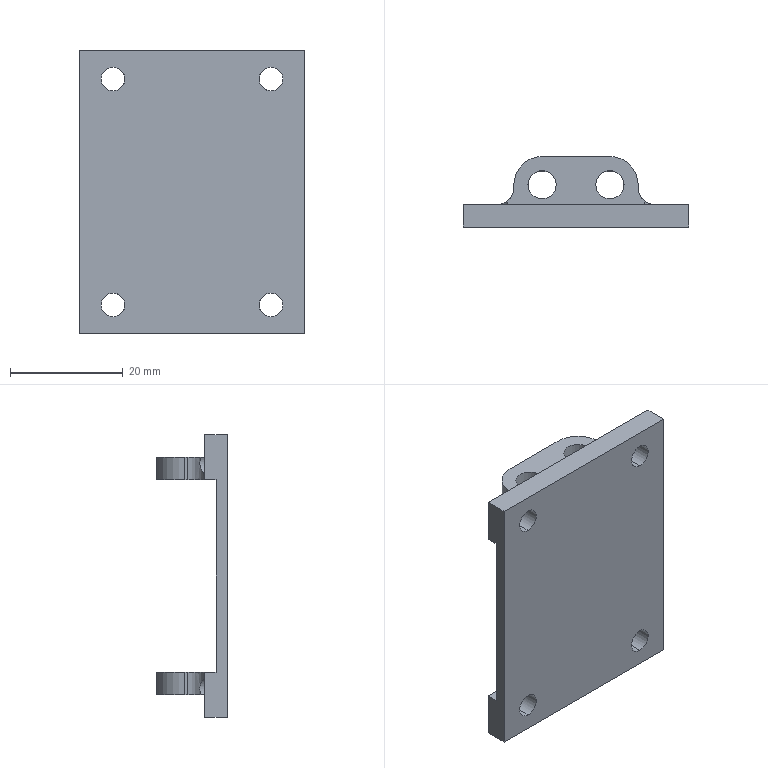Part | SolidWorks | features HoleWzd 3, ICE 3, Fillet 2, Extrusion 1 | 1 solid | 42 faces | box 40 x 12.5 x 50 mm | volume 6181 mm3 | cylinder 24 | plane 18 | commonest cylinder face diameters 4.2 x8 5 x8 6 x4 10 x4
STEP:
#1=CARTESIAN_POINT('',(2.5,0.,3.));
#2=VERTEX_POINT('',#1);
#3=CARTESIAN_POINT('',(-2.5,0.,3.));
#4=VERTEX_POINT('',#3);
#5=CARTESIAN_POINT('',(0.,0.,3.));
#6=DIRECTION('',(0.,0.,-1.));
#7=DIRECTION('',(-1.,0.,0.));
#8=AXIS2_PLACEMENT_3D('',#5,#6,#7);
#9=CIRCLE('',#8,2.5);
#10=EDGE_CURVE('',#2,#4,#9,.T.);
#11=ORIENTED_EDGE('',*,*,#10,.F.);
#12=CARTESIAN_POINT('',(2.5,0.,-1.));
#13=VERTEX_POINT('',#12);
#14=CARTESIAN_POINT('',(2.5,0.,-1.));
#15=DIRECTION('',(0.,0.,-1.));
#16=VECTOR('',#15,1000.);
#17=LINE('',#14,#16);
#18=EDGE_CURVE('',#2,#13,#17,.T.);
#19=ORIENTED_EDGE('',*,*,#18,.T.);
#20=CARTESIAN_POINT('',(-2.5,0.,-1.));
#21=VERTEX_POINT('',#20);
#22=CARTESIAN_POINT('',(0.,0.,-1.));
#23=DIRECTION('',(0.,0.,-1.));
#24=DIRECTION('',(-1.,0.,0.));
#25=AXIS2_PLACEMENT_3D('',#22,#23,#24);
#26=CIRCLE('',#25,2.5);
#27=EDGE_CURVE('',#13,#21,#26,.T.);
#28=ORIENTED_EDGE('',*,*,#27,.T.);
#29=CARTESIAN_POINT('',(-2.5,0.,-1.));
#30=DIRECTION('',(0.,0.,-1.));
#31=VECTOR('',#30,1000.);
#32=LINE('',#29,#31);
#33=EDGE_CURVE('',#4,#21,#32,.T.);
#34=ORIENTED_EDGE('',*,*,#33,.F.);
#35=EDGE_LOOP('',(#11,#19,#28,#34));
#36=FACE_OUTER_BOUND('',#35,.T.);
#37=CARTESIAN_POINT('',(0.,0.,-1.));
#38=DIRECTION('',(0.,0.,-1.));
#39=DIRECTION('',(-1.,0.,0.));
#40=AXIS2_PLACEMENT_3D('',#37,#38,#39);
#41=CYLINDRICAL_SURFACE('',#40,2.5);
#42=ADVANCED_FACE('',(#36),#41,.F.);
#43=CARTESIAN_POINT('',(14.5,0.,3.));
#44=VERTEX_POINT('',#43);
#45=CARTESIAN_POINT('',(9.5,0.,3.));
#46=VERTEX_POINT('',#45);
#47=CARTESIAN_POINT('',(12.,0.,3.));
#48=DIRECTION('',(0.,0.,-1.));
#49=DIRECTION('',(-1.,0.,0.));
#50=AXIS2_PLACEMENT_3D('',#47,#48,#49);
#51=CIRCLE('',#50,2.5);
#52=EDGE_CURVE('',#44,#46,#51,.T.);
#53=ORIENTED_EDGE('',*,*,#52,.F.);
#54=CARTESIAN_POINT('',(14.5,0.,-1.));
#55=VERTEX_POINT('',#54);
#56=CARTESIAN_POINT('',(14.5,0.,-1.));
#57=DIRECTION('',(0.,0.,-1.));
#58=VECTOR('',#57,1000.);
#59=LINE('',#56,#58);
#60=EDGE_CURVE('',#44,#55,#59,.T.);
#61=ORIENTED_EDGE('',*,*,#60,.T.);
#62=CARTESIAN_POINT('',(9.5,0.,-1.));
#63=VERTEX_POINT('',#62);
#64=CARTESIAN_POINT('',(12.,0.,-1.));
#65=DIRECTION('',(0.,0.,-1.));
#66=DIRECTION('',(-1.,0.,0.));
#67=AXIS2_PLACEMENT_3D('',#64,#65,#66);
#68=CIRCLE('',#67,2.5);
#69=EDGE_CURVE('',#55,#63,#68,.T.);
#70=ORIENTED_EDGE('',*,*,#69,.T.);
#71=CARTESIAN_POINT('',(9.5,0.,-1.));
#72=DIRECTION('',(0.,0.,-1.));
#73=VECTOR('',#72,1000.);
#74=LINE('',#71,#73);
#75=EDGE_CURVE('',#46,#63,#74,.T.);
#76=ORIENTED_EDGE('',*,*,#75,.F.);
#77=EDGE_LOOP('',(#53,#61,#70,#76));
#78=FACE_OUTER_BOUND('',#77,.T.);
#79=CARTESIAN_POINT('',(12.,0.,-1.));
#80=DIRECTION('',(0.,0.,-1.));
#81=DIRECTION('',(-1.,0.,0.));
#82=AXIS2_PLACEMENT_3D('',#79,#80,#81);
#83=CYLINDRICAL_SURFACE('',#82,2.5);
#84=ADVANCED_FACE('',(#78),#83,.F.);
#85=CARTESIAN_POINT('',(2.5,0.,41.));
#86=VERTEX_POINT('',#85);
#87=CARTESIAN_POINT('',(-2.5,0.,41.));
#88=VERTEX_POINT('',#87);
#89=CARTESIAN_POINT('',(0.,0.,41.));
#90=DIRECTION('',(0.,0.,-1.));
#91=DIRECTION('',(-1.,0.,0.));
#92=AXIS2_PLACEMENT_3D('',#89,#90,#91);
#93=CIRCLE('',#92,2.5);
#94=EDGE_CURVE('',#86,#88,#93,.T.);
#95=ORIENTED_EDGE('',*,*,#94,.F.);
#96=CARTESIAN_POINT('',(2.5,0.,37.));
#97=VERTEX_POINT('',#96);
#98=CARTESIAN_POINT('',(2.5,0.,37.));
#99=DIRECTION('',(0.,0.,-1.));
#100=VECTOR('',#99,1000.);
#101=LINE('',#98,#100);
#102=EDGE_CURVE('',#86,#97,#101,.T.);
#103=ORIENTED_EDGE('',*,*,#102,.T.);
#104=CARTESIAN_POINT('',(-2.5,0.,37.));
#105=VERTEX_POINT('',#104);
#106=CARTESIAN_POINT('',(0.,0.,37.));
#107=DIRECTION('',(0.,0.,-1.));
#108=DIRECTION('',(-1.,0.,0.));
#109=AXIS2_PLACEMENT_3D('',#106,#107,#108);
#110=CIRCLE('',#109,2.5);
#111=EDGE_CURVE('',#97,#105,#110,.T.);
#112=ORIENTED_EDGE('',*,*,#111,.T.);
#113=CARTESIAN_POINT('',(-2.5,0.,37.));
#114=DIRECTION('',(0.,0.,-1.));
#115=VECTOR('',#114,1000.);
#116=LINE('',#113,#115);
#117=EDGE_CURVE('',#88,#105,#116,.T.);
#118=ORIENTED_EDGE('',*,*,#117,.F.);
#119=EDGE_LOOP('',(#95,#103,#112,#118));
#120=FACE_OUTER_BOUND('',#119,.T.);
#121=CARTESIAN_POINT('',(0.,0.,37.));
#122=DIRECTION('',(0.,0.,-1.));
#123=DIRECTION('',(-1.,0.,0.));
#124=AXIS2_PLACEMENT_3D('',#121,#122,#123);
#125=CYLINDRICAL_SURFACE('',#124,2.5);
#126=ADVANCED_FACE('',(#120),#125,.F.);
#127=CARTESIAN_POINT('',(14.5,0.,41.));
#128=VERTEX_POINT('',#127);
#129=CARTESIAN_POINT('',(9.5,0.,41.));
#130=VERTEX_POINT('',#129);
#131=CARTESIAN_POINT('',(12.,0.,41.));
#132=DIRECTION('',(0.,0.,-1.));
#133=DIRECTION('',(-1.,0.,0.));
#134=AXIS2_PLACEMENT_3D('',#131,#132,#133);
#135=CIRCLE('',#134,2.5);
#136=EDGE_CURVE('',#128,#130,#135,.T.);
#137=ORIENTED_EDGE('',*,*,#136,.F.);
#138=CARTESIAN_POINT('',(14.5,0.,37.));
#139=VERTEX_POINT('',#138);
#140=CARTESIAN_POINT('',(14.5,0.,37.));
#141=DIRECTION('',(0.,0.,-1.));
#142=VECTOR('',#141,1000.);
#143=LINE('',#140,#142);
#144=EDGE_CURVE('',#128,#139,#143,.T.);
#145=ORIENTED_EDGE('',*,*,#144,.T.);
#146=CARTESIAN_POINT('',(9.5,0.,37.));
#147=VERTEX_POINT('',#146);
#148=CARTESIAN_POINT('',(12.,0.,37.));
#149=DIRECTION('',(0.,0.,-1.));
#150=DIRECTION('',(-1.,0.,0.));
#151=AXIS2_PLACEMENT_3D('',#148,#149,#150);
#152=CIRCLE('',#151,2.5);
#153=EDGE_CURVE('',#139,#147,#152,.T.);
#154=ORIENTED_EDGE('',*,*,#153,.T.);
#155=CARTESIAN_POINT('',(9.5,0.,37.));
#156=DIRECTION('',(0.,0.,-1.));
#157=VECTOR('',#156,1000.);
#158=LINE('',#155,#157);
#159=EDGE_CURVE('',#130,#147,#158,.T.);
#160=ORIENTED_EDGE('',*,*,#159,.F.);
#161=EDGE_LOOP('',(#137,#145,#154,#160));
#162=FACE_OUTER_BOUND('',#161,.T.);
#163=CARTESIAN_POINT('',(12.,0.,37.));
#164=DIRECTION('',(0.,0.,-1.));
#165=DIRECTION('',(-1.,0.,0.));
#166=AXIS2_PLACEMENT_3D('',#163,#164,#165);
#167=CYLINDRICAL_SURFACE('',#166,2.5);
#168=ADVANCED_FACE('',(#162),#167,.F.);
#169=CARTESIAN_POINT('',(18.153,-3.5,41.));
#170=VERTEX_POINT('',#169);
#171=CARTESIAN_POINT('',(20.,-3.5,42.1));
#172=VERTEX_POINT('',#171);
#173=CARTESIAN_POINT('',(20.,-3.5,40.));
#174=DIRECTION('',(0.,1.,0.));
#175=DIRECTION('',(0.,0.,1.));
#176=AXIS2_PLACEMENT_3D('',#173,#174,#175);
#177=CIRCLE('',#176,2.1);
#178=EDGE_CURVE('',#170,#172,#177,.T.);
#179=ORIENTED_EDGE('',*,*,#178,.T.);
#180=CARTESIAN_POINT('',(20.,-7.5,42.1));
#181=VERTEX_POINT('',#180);
#182=CARTESIAN_POINT('',(20.,-7.5,42.1));
#183=DIRECTION('',(0.,-1.,0.));
#184=VECTOR('',#183,1000.);
#185=LINE('',#182,#184);
#186=EDGE_CURVE('',#172,#181,#185,.T.);
#187=ORIENTED_EDGE('',*,*,#186,.T.);
#188=CARTESIAN_POINT('',(20.,-7.5,37.9));
#189=VERTEX_POINT('',#188);
#190=CARTESIAN_POINT('',(20.,-7.5,40.));
#191=DIRECTION('',(0.,-1.,0.));
#192=DIRECTION('',(0.,0.,-1.));
#193=AXIS2_PLACEMENT_3D('',#190,#191,#192);
#194=CIRCLE('',#193,2.1);
#195=EDGE_CURVE('',#181,#189,#194,.T.);
#196=ORIENTED_EDGE('',*,*,#195,.T.);
#197=CARTESIAN_POINT('',(20.,-3.5,37.9));
#198=VERTEX_POINT('',#197);
#199=CARTESIAN_POINT('',(20.,-7.5,37.9));
#200=DIRECTION('',(0.,-1.,0.));
#201=VECTOR('',#200,1000.);
#202=LINE('',#199,#201);
#203=EDGE_CURVE('',#198,#189,#202,.T.);
#204=ORIENTED_EDGE('',*,*,#203,.F.);
#205=CARTESIAN_POINT('',(18.153,-2.864,41.));
#206=VERTEX_POINT('',#205);
#207=CARTESIAN_POINT('',(20.,-3.5,37.9));
#208=CARTESIAN_POINT('',(19.811,-3.5,37.9));
#209=CARTESIAN_POINT('',(19.627,-3.482,37.925));
#210=CARTESIAN_POINT('',(19.269,-3.415,38.023));
#211=CARTESIAN_POINT('',(19.101,-3.367,38.094));
#212=CARTESIAN_POINT('',(18.638,-3.193,38.362));
#213=CARTESIAN_POINT('',(18.385,-3.038,38.614));
#214=CARTESIAN_POINT('',(18.115,-2.836,39.059));
#215=CARTESIAN_POINT('',(18.041,-2.773,39.222));
#216=CARTESIAN_POINT('',(17.963,-2.702,39.483));
#217=CARTESIAN_POINT('',(17.942,-2.683,39.573));
#218=CARTESIAN_POINT('',(17.912,-2.654,39.755));
#219=CARTESIAN_POINT('',(17.903,-2.646,39.85));
#220=CARTESIAN_POINT('',(17.896,-2.638,40.132));
#221=CARTESIAN_POINT('',(17.916,-2.659,40.319));
#222=CARTESIAN_POINT('',(18.004,-2.74,40.677));
#223=CARTESIAN_POINT('',(18.07,-2.799,40.845));
#224=CARTESIAN_POINT('',(18.153,-2.864,41.));
#225=B_SPLINE_CURVE_WITH_KNOTS('',3,(#207,#208,#209,#210,#211,#212,#213,#214,#215,#216,#217,#218,#219,#220,#221,#222,#223,#224),.UNSPECIFIED.,.F.,.F.,(4,2,2,2,2,2,2,2,4),(0.,0.0005592,0.001118,0.002237,0.002796,0.003076,0.003355,0.003915,0.004474),.UNSPECIFIED.);
#226=EDGE_CURVE('',#198,#206,#225,.T.);
#227=ORIENTED_EDGE('',*,*,#226,.T.);
#228=CARTESIAN_POINT('',(18.153,-2.864,41.));
#229=DIRECTION('',(0.,1.,0.));
#230=VECTOR('',#229,1000.);
#231=LINE('',#228,#230);
#232=EDGE_CURVE('',#170,#206,#231,.T.);
#233=ORIENTED_EDGE('',*,*,#232,.F.);
#234=EDGE_LOOP('',(#179,#187,#196,#204,#227,#233));
#235=FACE_OUTER_BOUND('',#234,.T.);
#236=CARTESIAN_POINT('',(20.,-7.5,40.));
#237=DIRECTION('',(0.,-1.,0.));
#238=DIRECTION('',(0.,0.,-1.));
#239=AXIS2_PLACEMENT_3D('',#236,#237,#238);
#240=CYLINDRICAL_SURFACE('',#239,2.1);
#241=ADVANCED_FACE('',(#235),#240,.F.);
#242=CARTESIAN_POINT('',(18.153,-2.864,-1.));
#243=VERTEX_POINT('',#242);
#244=CARTESIAN_POINT('',(20.,-3.5,2.1));
#245=VERTEX_POINT('',#244);
#246=CARTESIAN_POINT('',(18.153,-2.864,-1.));
#247=CARTESIAN_POINT('',(18.07,-2.799,-0.8455));
#248=CARTESIAN_POINT('',(18.004,-2.74,-0.6767));
#249=CARTESIAN_POINT('',(17.916,-2.659,-0.3194));
#250=CARTESIAN_POINT('',(17.896,-2.638,-0.1317));
#251=CARTESIAN_POINT('',(17.903,-2.646,0.15));
#252=CARTESIAN_POINT('',(17.912,-2.654,0.2446));
#253=CARTESIAN_POINT('',(17.942,-2.683,0.4274));
#254=CARTESIAN_POINT('',(17.963,-2.702,0.5166));
#255=CARTESIAN_POINT('',(18.041,-2.773,0.7784));
#256=CARTESIAN_POINT('',(18.115,-2.836,0.9408));
#257=CARTESIAN_POINT('',(18.385,-3.038,1.386));
#258=CARTESIAN_POINT('',(18.638,-3.193,1.638));
#259=CARTESIAN_POINT('',(19.101,-3.367,1.906));
#260=CARTESIAN_POINT('',(19.269,-3.415,1.977));
#261=CARTESIAN_POINT('',(19.627,-3.482,2.075));
#262=CARTESIAN_POINT('',(19.811,-3.5,2.1));
#263=CARTESIAN_POINT('',(20.,-3.5,2.1));
#264=B_SPLINE_CURVE_WITH_KNOTS('',3,(#246,#247,#248,#249,#250,#251,#252,#253,#254,#255,#256,#257,#258,#259,#260,#261,#262,#263),.UNSPECIFIED.,.F.,.F.,(4,2,2,2,2,2,2,2,4),(0.0006281,0.001188,0.001748,0.002027,0.002307,0.002867,0.003986,0.004546,0.005106),.UNSPECIFIED.);
#265=EDGE_CURVE('',#243,#245,#264,.T.);
#266=ORIENTED_EDGE('',*,*,#265,.T.);
#267=CARTESIAN_POINT('',(20.,-7.5,2.1));
#268=VERTEX_POINT('',#267);
#269=CARTESIAN_POINT('',(20.,-7.5,2.1));
#270=DIRECTION('',(0.,-1.,0.));
#271=VECTOR('',#270,1000.);
#272=LINE('',#269,#271);
#273=EDGE_CURVE('',#245,#268,#272,.T.);
#274=ORIENTED_EDGE('',*,*,#273,.T.);
#275=CARTESIAN_POINT('',(20.,-7.5,-2.1));
#276=VERTEX_POINT('',#275);
#277=CARTESIAN_POINT('',(20.,-7.5,0.));
#278=DIRECTION('',(0.,-1.,0.));
#279=DIRECTION('',(0.,0.,-1.));
#280=AXIS2_PLACEMENT_3D('',#277,#278,#279);
#281=CIRCLE('',#280,2.1);
#282=EDGE_CURVE('',#268,#276,#281,.T.);
#283=ORIENTED_EDGE('',*,*,#282,.T.);
#284=CARTESIAN_POINT('',(20.,-3.5,-2.1));
#285=VERTEX_POINT('',#284);
#286=CARTESIAN_POINT('',(20.,-7.5,-2.1));
#287=DIRECTION('',(0.,-1.,0.));
#288=VECTOR('',#287,1000.);
#289=LINE('',#286,#288);
#290=EDGE_CURVE('',#285,#276,#289,.T.);
#291=ORIENTED_EDGE('',*,*,#290,.F.);
#292=CARTESIAN_POINT('',(18.153,-3.5,-1.));
#293=VERTEX_POINT('',#292);
#294=CARTESIAN_POINT('',(20.,-3.5,0.));
#295=DIRECTION('',(0.,1.,0.));
#296=DIRECTION('',(0.,0.,1.));
#297=AXIS2_PLACEMENT_3D('',#294,#295,#296);
#298=CIRCLE('',#297,2.1);
#299=EDGE_CURVE('',#285,#293,#298,.T.);
#300=ORIENTED_EDGE('',*,*,#299,.T.);
#301=CARTESIAN_POINT('',(18.153,-3.5,-1.));
#302=DIRECTION('',(0.,1.,0.));
#303=VECTOR('',#302,1000.);
#304=LINE('',#301,#303);
#305=EDGE_CURVE('',#293,#243,#304,.T.);
#306=ORIENTED_EDGE('',*,*,#305,.T.);
#307=EDGE_LOOP('',(#266,#274,#283,#291,#300,#306));
#308=FACE_OUTER_BOUND('',#307,.T.);
#309=CARTESIAN_POINT('',(20.,-7.5,0.));
#310=DIRECTION('',(0.,-1.,0.));
#311=DIRECTION('',(0.,0.,-1.));
#312=AXIS2_PLACEMENT_3D('',#309,#310,#311);
#313=CYLINDRICAL_SURFACE('',#312,2.1);
#314=ADVANCED_FACE('',(#308),#313,.F.);
#315=CARTESIAN_POINT('',(-8.,-3.5,-2.1));
#316=VERTEX_POINT('',#315);
#317=CARTESIAN_POINT('',(-8.,-3.5,2.1));
#318=VERTEX_POINT('',#317);
#319=CARTESIAN_POINT('',(-8.,-3.5,0.));
#320=DIRECTION('',(0.,1.,0.));
#321=DIRECTION('',(0.,0.,1.));
#322=AXIS2_PLACEMENT_3D('',#319,#320,#321);
#323=CIRCLE('',#322,2.1);
#324=EDGE_CURVE('',#316,#318,#323,.T.);
#325=ORIENTED_EDGE('',*,*,#324,.T.);
#326=CARTESIAN_POINT('',(-8.,-7.5,2.1));
#327=VERTEX_POINT('',#326);
#328=CARTESIAN_POINT('',(-8.,-7.5,2.1));
#329=DIRECTION('',(0.,-1.,0.));
#330=VECTOR('',#329,1000.);
#331=LINE('',#328,#330);
#332=EDGE_CURVE('',#318,#327,#331,.T.);
#333=ORIENTED_EDGE('',*,*,#332,.T.);
#334=CARTESIAN_POINT('',(-8.,-7.5,-2.1));
#335=VERTEX_POINT('',#334);
#336=CARTESIAN_POINT('',(-8.,-7.5,0.));
#337=DIRECTION('',(0.,-1.,0.));
#338=DIRECTION('',(0.,0.,-1.));
#339=AXIS2_PLACEMENT_3D('',#336,#337,#338);
#340=CIRCLE('',#339,2.1);
#341=EDGE_CURVE('',#327,#335,#340,.T.);
#342=ORIENTED_EDGE('',*,*,#341,.T.);
#343=CARTESIAN_POINT('',(-8.,-7.5,-2.1));
#344=DIRECTION('',(0.,-1.,0.));
#345=VECTOR('',#344,1000.);
#346=LINE('',#343,#345);
#347=EDGE_CURVE('',#316,#335,#346,.T.);
#348=ORIENTED_EDGE('',*,*,#347,.F.);
#349=EDGE_LOOP('',(#325,#333,#342,#348));
#350=FACE_OUTER_BOUND('',#349,.T.);
#351=CARTESIAN_POINT('',(-8.,-7.5,0.));
#352=DIRECTION('',(0.,-1.,0.));
#353=DIRECTION('',(0.,0.,-1.));
#354=AXIS2_PLACEMENT_3D('',#351,#352,#353);
#355=CYLINDRICAL_SURFACE('',#354,2.1);
#356=ADVANCED_FACE('',(#350),#355,.F.);
#357=CARTESIAN_POINT('',(-8.,-3.5,37.9));
#358=VERTEX_POINT('',#357);
#359=CARTESIAN_POINT('',(-8.,-3.5,42.1));
#360=VERTEX_POINT('',#359);
#361=CARTESIAN_POINT('',(-8.,-3.5,40.));
#362=DIRECTION('',(0.,1.,0.));
#363=DIRECTION('',(0.,0.,1.));
#364=AXIS2_PLACEMENT_3D('',#361,#362,#363);
#365=CIRCLE('',#364,2.1);
#366=EDGE_CURVE('',#358,#360,#365,.T.);
#367=ORIENTED_EDGE('',*,*,#366,.T.);
#368=CARTESIAN_POINT('',(-8.,-7.5,42.1));
#369=VERTEX_POINT('',#368);
#370=CARTESIAN_POINT('',(-8.,-7.5,42.1));
#371=DIRECTION('',(0.,-1.,0.));
#372=VECTOR('',#371,1000.);
#373=LINE('',#370,#372);
#374=EDGE_CURVE('',#360,#369,#373,.T.);
#375=ORIENTED_EDGE('',*,*,#374,.T.);
#376=CARTESIAN_POINT('',(-8.,-7.5,37.9));
#377=VERTEX_POINT('',#376);
#378=CARTESIAN_POINT('',(-8.,-7.5,40.));
#379=DIRECTION('',(0.,-1.,0.));
#380=DIRECTION('',(0.,0.,-1.));
#381=AXIS2_PLACEMENT_3D('',#378,#379,#380);
#382=CIRCLE('',#381,2.1);
#383=EDGE_CURVE('',#369,#377,#382,.T.);
#384=ORIENTED_EDGE('',*,*,#383,.T.);
#385=CARTESIAN_POINT('',(-8.,-7.5,37.9));
#386=DIRECTION('',(0.,-1.,0.));
#387=VECTOR('',#386,1000.);
#388=LINE('',#385,#387);
#389=EDGE_CURVE('',#358,#377,#388,.T.);
#390=ORIENTED_EDGE('',*,*,#389,.F.);
#391=EDGE_LOOP('',(#367,#375,#384,#390));
#392=FACE_OUTER_BOUND('',#391,.T.);
#393=CARTESIAN_POINT('',(-8.,-7.5,40.));
#394=DIRECTION('',(0.,-1.,0.));
#395=DIRECTION('',(0.,0.,-1.));
#396=AXIS2_PLACEMENT_3D('',#393,#394,#395);
#397=CYLINDRICAL_SURFACE('',#396,2.1);
#398=ADVANCED_FACE('',(#392),#397,.F.);
#399=CARTESIAN_POINT('',(-6.153,-3.5,41.));
#400=VERTEX_POINT('',#399);
#401=CARTESIAN_POINT('',(17.,-3.5,41.));
#402=DIRECTION('',(1.,0.,0.));
#403=VECTOR('',#402,1000.);
#404=LINE('',#401,#403);
#405=EDGE_CURVE('',#400,#170,#404,.T.);
#406=ORIENTED_EDGE('',*,*,#405,.F.);
#407=CARTESIAN_POINT('',(-8.,-3.5,40.));
#408=DIRECTION('',(0.,1.,0.));
#409=DIRECTION('',(0.,0.,1.));
#410=AXIS2_PLACEMENT_3D('',#407,#408,#409);
#411=CIRCLE('',#410,2.1);
#412=EDGE_CURVE('',#360,#400,#411,.T.);
#413=ORIENTED_EDGE('',*,*,#412,.F.);
#414=ORIENTED_EDGE('',*,*,#366,.F.);
#415=CARTESIAN_POINT('',(-8.,-3.5,37.));
#416=VERTEX_POINT('',#415);
#417=CARTESIAN_POINT('',(-8.,-3.5,0.));
#418=DIRECTION('',(0.,0.,-1.));
#419=VECTOR('',#418,1000.);
#420=LINE('',#417,#419);
#421=EDGE_CURVE('',#358,#416,#420,.T.);
#422=ORIENTED_EDGE('',*,*,#421,.T.);
#423=CARTESIAN_POINT('',(-14.,-3.5,37.));
#424=VERTEX_POINT('',#423);
#425=CARTESIAN_POINT('',(-14.,-3.5,37.));
#426=DIRECTION('',(1.,0.,0.));
#427=VECTOR('',#426,1000.);
#428=LINE('',#425,#427);
#429=EDGE_CURVE('',#424,#416,#428,.T.);
#430=ORIENTED_EDGE('',*,*,#429,.F.);
#431=CARTESIAN_POINT('',(-14.,-3.5,45.));
#432=VERTEX_POINT('',#431);
#433=CARTESIAN_POINT('',(-14.,-3.5,-5.));
#434=DIRECTION('',(0.,0.,1.));
#435=VECTOR('',#434,1000.);
#436=LINE('',#433,#435);
#437=EDGE_CURVE('',#424,#432,#436,.T.);
#438=ORIENTED_EDGE('',*,*,#437,.T.);
#439=CARTESIAN_POINT('',(26.,-3.5,45.));
#440=VERTEX_POINT('',#439);
#441=CARTESIAN_POINT('',(-14.,-3.5,45.));
#442=DIRECTION('',(1.,0.,0.));
#443=VECTOR('',#442,1000.);
#444=LINE('',#441,#443);
#445=EDGE_CURVE('',#432,#440,#444,.T.);
#446=ORIENTED_EDGE('',*,*,#445,.T.);
#447=CARTESIAN_POINT('',(26.,-3.5,37.));
#448=VERTEX_POINT('',#447);
#449=CARTESIAN_POINT('',(26.,-3.5,45.));
#450=DIRECTION('',(0.,0.,-1.));
#451=VECTOR('',#450,1000.);
#452=LINE('',#449,#451);
#453=EDGE_CURVE('',#440,#448,#452,.T.);
#454=ORIENTED_EDGE('',*,*,#453,.T.);
#455=CARTESIAN_POINT('',(20.,-3.5,37.));
#456=VERTEX_POINT('',#455);
#457=CARTESIAN_POINT('',(-14.,-3.5,37.));
#458=DIRECTION('',(1.,0.,0.));
#459=VECTOR('',#458,1000.);
#460=LINE('',#457,#459);
#461=EDGE_CURVE('',#456,#448,#460,.T.);
#462=ORIENTED_EDGE('',*,*,#461,.F.);
#463=CARTESIAN_POINT('',(20.,-3.5,0.));
#464=DIRECTION('',(0.,0.,1.));
#465=VECTOR('',#464,1000.);
#466=LINE('',#463,#465);
#467=EDGE_CURVE('',#456,#198,#466,.T.);
#468=ORIENTED_EDGE('',*,*,#467,.T.);
#469=CARTESIAN_POINT('',(20.,-3.5,40.));
#470=DIRECTION('',(0.,1.,0.));
#471=DIRECTION('',(0.,0.,1.));
#472=AXIS2_PLACEMENT_3D('',#469,#470,#471);
#473=CIRCLE('',#472,2.1);
#474=EDGE_CURVE('',#172,#198,#473,.T.);
#475=ORIENTED_EDGE('',*,*,#474,.F.);
#476=ORIENTED_EDGE('',*,*,#178,.F.);
#477=EDGE_LOOP('',(#406,#413,#414,#422,#430,#438,#446,#454,#462,#468,#475,#476));
#478=FACE_OUTER_BOUND('',#477,.T.);
#479=CARTESIAN_POINT('',(0.,-3.5,0.));
#480=DIRECTION('',(0.,1.,0.));
#481=DIRECTION('',(0.,0.,1.));
#482=AXIS2_PLACEMENT_3D('',#479,#480,#481);
#483=PLANE('',#482);
#484=ADVANCED_FACE('',(#478),#483,.T.);
#485=CARTESIAN_POINT('',(-14.,-3.5,3.));
#486=VERTEX_POINT('',#485);
#487=CARTESIAN_POINT('',(-8.,-3.5,3.));
#488=VERTEX_POINT('',#487);
#489=CARTESIAN_POINT('',(-14.,-3.5,3.));
#490=DIRECTION('',(1.,0.,0.));
#491=VECTOR('',#490,1000.);
#492=LINE('',#489,#491);
#493=EDGE_CURVE('',#486,#488,#492,.T.);
#494=ORIENTED_EDGE('',*,*,#493,.T.);
#495=CARTESIAN_POINT('',(-8.,-3.5,0.));
#496=DIRECTION('',(0.,0.,-1.));
#497=VECTOR('',#496,1000.);
#498=LINE('',#495,#497);
#499=EDGE_CURVE('',#488,#318,#498,.T.);
#500=ORIENTED_EDGE('',*,*,#499,.T.);
#501=ORIENTED_EDGE('',*,*,#324,.F.);
#502=CARTESIAN_POINT('',(-6.153,-3.5,-1.));
#503=VERTEX_POINT('',#502);
#504=CARTESIAN_POINT('',(-8.,-3.5,0.));
#505=DIRECTION('',(0.,1.,0.));
#506=DIRECTION('',(0.,0.,1.));
#507=AXIS2_PLACEMENT_3D('',#504,#505,#506);
#508=CIRCLE('',#507,2.1);
#509=EDGE_CURVE('',#503,#316,#508,.T.);
#510=ORIENTED_EDGE('',*,*,#509,.F.);
#511=CARTESIAN_POINT('',(-5.,-3.5,-1.));
#512=DIRECTION('',(-1.,0.,0.));
#513=VECTOR('',#512,1000.);
#514=LINE('',#511,#513);
#515=EDGE_CURVE('',#293,#503,#514,.T.);
#516=ORIENTED_EDGE('',*,*,#515,.F.);
#517=ORIENTED_EDGE('',*,*,#299,.F.);
#518=CARTESIAN_POINT('',(20.,-3.5,0.));
#519=DIRECTION('',(0.,1.,0.));
#520=DIRECTION('',(0.,0.,1.));
#521=AXIS2_PLACEMENT_3D('',#518,#519,#520);
#522=CIRCLE('',#521,2.1);
#523=EDGE_CURVE('',#245,#285,#522,.T.);
#524=ORIENTED_EDGE('',*,*,#523,.F.);
#525=CARTESIAN_POINT('',(20.,-3.5,3.));
#526=VERTEX_POINT('',#525);
#527=CARTESIAN_POINT('',(20.,-3.5,0.));
#528=DIRECTION('',(0.,0.,1.));
#529=VECTOR('',#528,1000.);
#530=LINE('',#527,#529);
#531=EDGE_CURVE('',#245,#526,#530,.T.);
#532=ORIENTED_EDGE('',*,*,#531,.T.);
#533=CARTESIAN_POINT('',(26.,-3.5,3.));
#534=VERTEX_POINT('',#533);
#535=CARTESIAN_POINT('',(-14.,-3.5,3.));
#536=DIRECTION('',(1.,0.,0.));
#537=VECTOR('',#536,1000.);
#538=LINE('',#535,#537);
#539=EDGE_CURVE('',#526,#534,#538,.T.);
#540=ORIENTED_EDGE('',*,*,#539,.T.);
#541=CARTESIAN_POINT('',(26.,-3.5,-5.));
#542=VERTEX_POINT('',#541);
#543=CARTESIAN_POINT('',(26.,-3.5,45.));
#544=DIRECTION('',(0.,0.,-1.));
#545=VECTOR('',#544,1000.);
#546=LINE('',#543,#545);
#547=EDGE_CURVE('',#534,#542,#546,.T.);
#548=ORIENTED_EDGE('',*,*,#547,.T.);
#549=CARTESIAN_POINT('',(-14.,-3.5,-5.));
#550=VERTEX_POINT('',#549);
#551=CARTESIAN_POINT('',(26.,-3.5,-5.));
#552=DIRECTION('',(-1.,0.,0.));
#553=VECTOR('',#552,1000.);
#554=LINE('',#551,#553);
#555=EDGE_CURVE('',#542,#550,#554,.T.);
#556=ORIENTED_EDGE('',*,*,#555,.T.);
#557=CARTESIAN_POINT('',(-14.,-3.5,-5.));
#558=DIRECTION('',(0.,0.,1.));
#559=VECTOR('',#558,1000.);
#560=LINE('',#557,#559);
#561=EDGE_CURVE('',#550,#486,#560,.T.);
#562=ORIENTED_EDGE('',*,*,#561,.T.);
#563=EDGE_LOOP('',(#494,#500,#501,#510,#516,#517,#524,#532,#540,#548,#556,#562));
#564=FACE_OUTER_BOUND('',#563,.T.);
#565=CARTESIAN_POINT('',(0.,-3.5,0.));
#566=DIRECTION('',(0.,1.,0.));
#567=DIRECTION('',(0.,0.,1.));
#568=AXIS2_PLACEMENT_3D('',#565,#566,#567);
#569=PLANE('',#568);
#570=ADVANCED_FACE('',(#564),#569,.T.);
#571=CARTESIAN_POINT('',(-14.,-5.5,3.));
#572=VERTEX_POINT('',#571);
#573=CARTESIAN_POINT('',(-14.,-5.5,3.));
#574=DIRECTION('',(0.,1.,0.));
#575=VECTOR('',#574,1000.);
#576=LINE('',#573,#575);
#577=EDGE_CURVE('',#572,#486,#576,.T.);
#578=ORIENTED_EDGE('',*,*,#577,.T.);
#579=ORIENTED_EDGE('',*,*,#561,.F.);
#580=CARTESIAN_POINT('',(-14.,-7.5,-5.));
#581=VERTEX_POINT('',#580);
#582=CARTESIAN_POINT('',(-14.,-7.5,-5.));
#583=DIRECTION('',(0.,1.,0.));
#584=VECTOR('',#583,1000.);
#585=LINE('',#582,#584);
#586=EDGE_CURVE('',#581,#550,#585,.T.);
#587=ORIENTED_EDGE('',*,*,#586,.F.);
#588=CARTESIAN_POINT('',(-14.,-7.5,45.));
#589=VERTEX_POINT('',#588);
#590=CARTESIAN_POINT('',(-14.,-7.5,-5.));
#591=DIRECTION('',(0.,0.,1.));
#592=VECTOR('',#591,1000.);
#593=LINE('',#590,#592);
#594=EDGE_CURVE('',#581,#589,#593,.T.);
#595=ORIENTED_EDGE('',*,*,#594,.T.);
#596=CARTESIAN_POINT('',(-14.,-7.5,45.));
#597=DIRECTION('',(0.,1.,0.));
#598=VECTOR('',#597,1000.);
#599=LINE('',#596,#598);
#600=EDGE_CURVE('',#589,#432,#599,.T.);
#601=ORIENTED_EDGE('',*,*,#600,.T.);
#602=ORIENTED_EDGE('',*,*,#437,.F.);
#603=CARTESIAN_POINT('',(-14.,-5.5,37.));
#604=VERTEX_POINT('',#603);
#605=CARTESIAN_POINT('',(-14.,-3.5,37.));
#606=DIRECTION('',(0.,-1.,0.));
#607=VECTOR('',#606,1000.);
#608=LINE('',#605,#607);
#609=EDGE_CURVE('',#424,#604,#608,.T.);
#610=ORIENTED_EDGE('',*,*,#609,.T.);
#611=CARTESIAN_POINT('',(-14.,-5.5,37.));
#612=DIRECTION('',(0.,0.,-1.));
#613=VECTOR('',#612,1000.);
#614=LINE('',#611,#613);
#615=EDGE_CURVE('',#604,#572,#614,.T.);
#616=ORIENTED_EDGE('',*,*,#615,.T.);
#617=EDGE_LOOP('',(#578,#579,#587,#595,#601,#602,#610,#616));
#618=FACE_OUTER_BOUND('',#617,.T.);
#619=CARTESIAN_POINT('',(-14.,-7.5,-5.));
#620=DIRECTION('',(-1.,0.,0.));
#621=DIRECTION('',(0.,0.,1.));
#622=AXIS2_PLACEMENT_3D('',#619,#620,#621);
#623=PLANE('',#622);
#624=ADVANCED_FACE('',(#618),#623,.T.);
#625=ORIENTED_EDGE('',*,*,#555,.F.);
#626=CARTESIAN_POINT('',(26.,-7.5,-5.));
#627=VERTEX_POINT('',#626);
#628=CARTESIAN_POINT('',(26.,-7.5,-5.));
#629=DIRECTION('',(0.,1.,0.));
#630=VECTOR('',#629,1000.);
#631=LINE('',#628,#630);
#632=EDGE_CURVE('',#627,#542,#631,.T.);
#633=ORIENTED_EDGE('',*,*,#632,.F.);
#634=CARTESIAN_POINT('',(26.,-7.5,-5.));
#635=DIRECTION('',(-1.,0.,0.));
#636=VECTOR('',#635,1000.);
#637=LINE('',#634,#636);
#638=EDGE_CURVE('',#627,#581,#637,.T.);
#639=ORIENTED_EDGE('',*,*,#638,.T.);
#640=ORIENTED_EDGE('',*,*,#586,.T.);
#641=EDGE_LOOP('',(#625,#633,#639,#640));
#642=FACE_OUTER_BOUND('',#641,.T.);
#643=CARTESIAN_POINT('',(26.,-7.5,-5.));
#644=DIRECTION('',(0.,0.,-1.));
#645=DIRECTION('',(-1.,0.,0.));
#646=AXIS2_PLACEMENT_3D('',#643,#644,#645);
#647=PLANE('',#646);
#648=ADVANCED_FACE('',(#642),#647,.T.);
#649=CARTESIAN_POINT('',(26.,-5.5,3.));
#650=VERTEX_POINT('',#649);
#651=CARTESIAN_POINT('',(26.,-5.5,3.));
#652=DIRECTION('',(0.,1.,0.));
#653=VECTOR('',#652,1000.);
#654=LINE('',#651,#653);
#655=EDGE_CURVE('',#650,#534,#654,.T.);
#656=ORIENTED_EDGE('',*,*,#655,.F.);
#657=CARTESIAN_POINT('',(26.,-5.5,37.));
#658=VERTEX_POINT('',#657);
#659=CARTESIAN_POINT('',(26.,-5.5,37.));
#660=DIRECTION('',(0.,0.,-1.));
#661=VECTOR('',#660,1000.);
#662=LINE('',#659,#661);
#663=EDGE_CURVE('',#658,#650,#662,.T.);
#664=ORIENTED_EDGE('',*,*,#663,.F.);
#665=CARTESIAN_POINT('',(26.,-3.5,37.));
#666=DIRECTION('',(0.,-1.,0.));
#667=VECTOR('',#666,1000.);
#668=LINE('',#665,#667);
#669=EDGE_CURVE('',#448,#658,#668,.T.);
#670=ORIENTED_EDGE('',*,*,#669,.F.);
#671=ORIENTED_EDGE('',*,*,#453,.F.);
#672=CARTESIAN_POINT('',(26.,-7.5,45.));
#673=VERTEX_POINT('',#672);
#674=CARTESIAN_POINT('',(26.,-7.5,45.));
#675=DIRECTION('',(0.,1.,0.));
#676=VECTOR('',#675,1000.);
#677=LINE('',#674,#676);
#678=EDGE_CURVE('',#673,#440,#677,.T.);
#679=ORIENTED_EDGE('',*,*,#678,.F.);
#680=CARTESIAN_POINT('',(26.,-7.5,45.));
#681=DIRECTION('',(0.,0.,-1.));
#682=VECTOR('',#681,1000.);
#683=LINE('',#680,#682);
#684=EDGE_CURVE('',#673,#627,#683,.T.);
#685=ORIENTED_EDGE('',*,*,#684,.T.);
#686=ORIENTED_EDGE('',*,*,#632,.T.);
#687=ORIENTED_EDGE('',*,*,#547,.F.);
#688=EDGE_LOOP('',(#656,#664,#670,#671,#679,#685,#686,#687));
#689=FACE_OUTER_BOUND('',#688,.T.);
#690=CARTESIAN_POINT('',(26.,-7.5,45.));
#691=DIRECTION('',(1.,0.,0.));
#692=DIRECTION('',(0.,0.,-1.));
#693=AXIS2_PLACEMENT_3D('',#690,#691,#692);
#694=PLANE('',#693);
#695=ADVANCED_FACE('',(#689),#694,.T.);
#696=ORIENTED_EDGE('',*,*,#445,.F.);
#697=ORIENTED_EDGE('',*,*,#600,.F.);
#698=CARTESIAN_POINT('',(-14.,-7.5,45.));
#699=DIRECTION('',(1.,0.,0.));
#700=VECTOR('',#699,1000.);
#701=LINE('',#698,#700);
#702=EDGE_CURVE('',#589,#673,#701,.T.);
#703=ORIENTED_EDGE('',*,*,#702,.T.);
#704=ORIENTED_EDGE('',*,*,#678,.T.);
#705=EDGE_LOOP('',(#696,#697,#703,#704));
#706=FACE_OUTER_BOUND('',#705,.T.);
#707=CARTESIAN_POINT('',(-14.,-7.5,45.));
#708=DIRECTION('',(0.,0.,1.));
#709=DIRECTION('',(1.,0.,0.));
#710=AXIS2_PLACEMENT_3D('',#707,#708,#709);
#711=PLANE('',#710);
#712=ADVANCED_FACE('',(#706),#711,.T.);
#713=CARTESIAN_POINT('',(20.,-7.5,40.));
#714=DIRECTION('',(0.,-1.,0.));
#715=DIRECTION('',(0.,0.,-1.));
#716=AXIS2_PLACEMENT_3D('',#713,#714,#715);
#717=CIRCLE('',#716,2.1);
#718=EDGE_CURVE('',#189,#181,#717,.T.);
#719=ORIENTED_EDGE('',*,*,#718,.F.);
#720=ORIENTED_EDGE('',*,*,#195,.F.);
#721=EDGE_LOOP('',(#719,#720));
#722=FACE_BOUND('',#721,.T.);
#723=CARTESIAN_POINT('',(20.,-7.5,0.));
#724=DIRECTION('',(0.,-1.,0.));
#725=DIRECTION('',(0.,0.,-1.));
#726=AXIS2_PLACEMENT_3D('',#723,#724,#725);
#727=CIRCLE('',#726,2.1);
#728=EDGE_CURVE('',#276,#268,#727,.T.);
#729=ORIENTED_EDGE('',*,*,#728,.F.);
#730=ORIENTED_EDGE('',*,*,#282,.F.);
#731=EDGE_LOOP('',(#729,#730));
#732=FACE_BOUND('',#731,.T.);
#733=CARTESIAN_POINT('',(-8.,-7.5,0.));
#734=DIRECTION('',(0.,-1.,0.));
#735=DIRECTION('',(0.,0.,-1.));
#736=AXIS2_PLACEMENT_3D('',#733,#734,#735);
#737=CIRCLE('',#736,2.1);
#738=EDGE_CURVE('',#335,#327,#737,.T.);
#739=ORIENTED_EDGE('',*,*,#738,.F.);
#740=ORIENTED_EDGE('',*,*,#341,.F.);
#741=EDGE_LOOP('',(#739,#740));
#742=FACE_BOUND('',#741,.T.);
#743=CARTESIAN_POINT('',(-8.,-7.5,40.));
#744=DIRECTION('',(0.,-1.,0.));
#745=DIRECTION('',(0.,0.,-1.));
#746=AXIS2_PLACEMENT_3D('',#743,#744,#745);
#747=CIRCLE('',#746,2.1);
#748=EDGE_CURVE('',#377,#369,#747,.T.);
#749=ORIENTED_EDGE('',*,*,#748,.F.);
#750=ORIENTED_EDGE('',*,*,#383,.F.);
#751=EDGE_LOOP('',(#749,#750));
#752=FACE_BOUND('',#751,.T.);
#753=ORIENTED_EDGE('',*,*,#594,.F.);
#754=ORIENTED_EDGE('',*,*,#638,.F.);
#755=ORIENTED_EDGE('',*,*,#684,.F.);
#756=ORIENTED_EDGE('',*,*,#702,.F.);
#757=EDGE_LOOP('',(#753,#754,#755,#756));
#758=FACE_OUTER_BOUND('',#757,.T.);
#759=CARTESIAN_POINT('',(0.,-7.5,0.));
#760=DIRECTION('',(0.,1.,0.));
#761=DIRECTION('',(0.,0.,1.));
#762=AXIS2_PLACEMENT_3D('',#759,#760,#761);
#763=PLANE('',#762);
#764=ADVANCED_FACE('',(#722,#732,#742,#752,#758),#763,.F.);
#765=CARTESIAN_POINT('',(0.,0.,3.));
#766=DIRECTION('',(0.,0.,-1.));
#767=DIRECTION('',(-1.,0.,0.));
#768=AXIS2_PLACEMENT_3D('',#765,#766,#767);
#769=CIRCLE('',#768,2.5);
#770=EDGE_CURVE('',#4,#2,#769,.T.);
#771=ORIENTED_EDGE('',*,*,#770,.T.);
#772=ORIENTED_EDGE('',*,*,#10,.T.);
#773=EDGE_LOOP('',(#771,#772));
#774=FACE_BOUND('',#773,.T.);
#775=CARTESIAN_POINT('',(12.,0.,3.));
#776=DIRECTION('',(0.,0.,-1.));
#777=DIRECTION('',(-1.,0.,0.));
#778=AXIS2_PLACEMENT_3D('',#775,#776,#777);
#779=CIRCLE('',#778,2.5);
#780=EDGE_CURVE('',#46,#44,#779,.T.);
#781=ORIENTED_EDGE('',*,*,#780,.T.);
#782=ORIENTED_EDGE('',*,*,#52,.T.);
#783=EDGE_LOOP('',(#781,#782));
#784=FACE_BOUND('',#783,.T.);
#785=CARTESIAN_POINT('',(0.,5.,3.));
#786=VERTEX_POINT('',#785);
#787=CARTESIAN_POINT('',(12.,5.,3.));
#788=VERTEX_POINT('',#787);
#789=CARTESIAN_POINT('',(17.,5.,3.));
#790=DIRECTION('',(1.,0.,0.));
#791=VECTOR('',#790,1000.);
#792=LINE('',#789,#791);
#793=EDGE_CURVE('',#786,#788,#792,.T.);
#794=ORIENTED_EDGE('',*,*,#793,.F.);
#795=CARTESIAN_POINT('',(-5.,0.,3.));
#796=VERTEX_POINT('',#795);
#797=CARTESIAN_POINT('',(0.,0.,3.));
#798=DIRECTION('',(0.,0.,1.));
#799=DIRECTION('',(-1.,0.,0.));
#800=AXIS2_PLACEMENT_3D('',#797,#798,#799);
#801=CIRCLE('',#800,5.);
#802=EDGE_CURVE('',#786,#796,#801,.T.);
#803=ORIENTED_EDGE('',*,*,#802,.T.);
#804=CARTESIAN_POINT('',(-5.,-0.5,3.));
#805=VERTEX_POINT('',#804);
#806=CARTESIAN_POINT('',(-5.,5.,3.));
#807=DIRECTION('',(0.,-1.,0.));
#808=VECTOR('',#807,1000.);
#809=LINE('',#806,#808);
#810=EDGE_CURVE('',#796,#805,#809,.T.);
#811=ORIENTED_EDGE('',*,*,#810,.T.);
#812=CARTESIAN_POINT('',(-8.,-0.5,3.));
#813=DIRECTION('',(0.,0.,-1.));
#814=DIRECTION('',(-1.,0.,0.));
#815=AXIS2_PLACEMENT_3D('',#812,#813,#814);
#816=CIRCLE('',#815,3.);
#817=EDGE_CURVE('',#805,#488,#816,.T.);
#818=ORIENTED_EDGE('',*,*,#817,.T.);
#819=ORIENTED_EDGE('',*,*,#493,.F.);
#820=ORIENTED_EDGE('',*,*,#577,.F.);
#821=CARTESIAN_POINT('',(-14.,-5.5,3.));
#822=DIRECTION('',(1.,0.,0.));
#823=VECTOR('',#822,1000.);
#824=LINE('',#821,#823);
#825=EDGE_CURVE('',#572,#650,#824,.T.);
#826=ORIENTED_EDGE('',*,*,#825,.T.);
#827=ORIENTED_EDGE('',*,*,#655,.T.);
#828=ORIENTED_EDGE('',*,*,#539,.F.);
#829=CARTESIAN_POINT('',(17.,-0.5,3.));
#830=VERTEX_POINT('',#829);
#831=CARTESIAN_POINT('',(20.,-0.5,3.));
#832=DIRECTION('',(0.,0.,-1.));
#833=DIRECTION('',(-1.,0.,0.));
#834=AXIS2_PLACEMENT_3D('',#831,#832,#833);
#835=CIRCLE('',#834,3.);
#836=EDGE_CURVE('',#526,#830,#835,.T.);
#837=ORIENTED_EDGE('',*,*,#836,.T.);
#838=CARTESIAN_POINT('',(17.,0.,3.));
#839=VERTEX_POINT('',#838);
#840=CARTESIAN_POINT('',(17.,5.,3.));
#841=DIRECTION('',(0.,-1.,0.));
#842=VECTOR('',#841,1000.);
#843=LINE('',#840,#842);
#844=EDGE_CURVE('',#839,#830,#843,.T.);
#845=ORIENTED_EDGE('',*,*,#844,.F.);
#846=CARTESIAN_POINT('',(12.,0.,3.));
#847=DIRECTION('',(0.,0.,1.));
#848=DIRECTION('',(-1.,0.,0.));
#849=AXIS2_PLACEMENT_3D('',#846,#847,#848);
#850=CIRCLE('',#849,5.);
#851=EDGE_CURVE('',#839,#788,#850,.T.);
#852=ORIENTED_EDGE('',*,*,#851,.T.);
#853=EDGE_LOOP('',(#794,#803,#811,#818,#819,#820,#826,#827,#828,#837,#845,#852));
#854=FACE_OUTER_BOUND('',#853,.T.);
#855=CARTESIAN_POINT('',(-14.,-5.5,3.));
#856=DIRECTION('',(0.,0.,-1.));
#857=DIRECTION('',(-1.,0.,0.));
#858=AXIS2_PLACEMENT_3D('',#855,#856,#857);
#859=PLANE('',#858);
#860=ADVANCED_FACE('',(#774,#784,#854),#859,.F.);
#861=ORIENTED_EDGE('',*,*,#663,.T.);
#862=ORIENTED_EDGE('',*,*,#825,.F.);
#863=ORIENTED_EDGE('',*,*,#615,.F.);
#864=CARTESIAN_POINT('',(-14.,-5.5,37.));
#865=DIRECTION('',(1.,0.,0.));
#866=VECTOR('',#865,1000.);
#867=LINE('',#864,#866);
#868=EDGE_CURVE('',#604,#658,#867,.T.);
#869=ORIENTED_EDGE('',*,*,#868,.T.);
#870=EDGE_LOOP('',(#861,#862,#863,#869));
#871=FACE_OUTER_BOUND('',#870,.T.);
#872=CARTESIAN_POINT('',(-14.,-5.5,37.));
#873=DIRECTION('',(0.,-1.,0.));
#874=DIRECTION('',(0.,0.,-1.));
#875=AXIS2_PLACEMENT_3D('',#872,#873,#874);
#876=PLANE('',#875);
#877=ADVANCED_FACE('',(#871),#876,.F.);
#878=CARTESIAN_POINT('',(0.,0.,37.));
#879=DIRECTION('',(0.,0.,-1.));
#880=DIRECTION('',(-1.,0.,0.));
#881=AXIS2_PLACEMENT_3D('',#878,#879,#880);
#882=CIRCLE('',#881,2.5);
#883=EDGE_CURVE('',#105,#97,#882,.T.);
#884=ORIENTED_EDGE('',*,*,#883,.F.);
#885=ORIENTED_EDGE('',*,*,#111,.F.);
#886=EDGE_LOOP('',(#884,#885));
#887=FACE_BOUND('',#886,.T.);
#888=CARTESIAN_POINT('',(12.,0.,37.));
#889=DIRECTION('',(0.,0.,-1.));
#890=DIRECTION('',(-1.,0.,0.));
#891=AXIS2_PLACEMENT_3D('',#888,#889,#890);
#892=CIRCLE('',#891,2.5);
#893=EDGE_CURVE('',#147,#139,#892,.T.);
#894=ORIENTED_EDGE('',*,*,#893,.F.);
#895=ORIENTED_EDGE('',*,*,#153,.F.);
#896=EDGE_LOOP('',(#894,#895));
#897=FACE_BOUND('',#896,.T.);
#898=CARTESIAN_POINT('',(-5.,0.,37.));
#899=VERTEX_POINT('',#898);
#900=CARTESIAN_POINT('',(-5.,-0.5,37.));
#901=VERTEX_POINT('',#900);
#902=CARTESIAN_POINT('',(-5.,5.,37.));
#903=DIRECTION('',(0.,-1.,0.));
#904=VECTOR('',#903,1000.);
#905=LINE('',#902,#904);
#906=EDGE_CURVE('',#899,#901,#905,.T.);
#907=ORIENTED_EDGE('',*,*,#906,.F.);
#908=CARTESIAN_POINT('',(0.,5.,37.));
#909=VERTEX_POINT('',#908);
#910=CARTESIAN_POINT('',(0.,0.,37.));
#911=DIRECTION('',(0.,0.,-1.));
#912=DIRECTION('',(1.,0.,0.));
#913=AXIS2_PLACEMENT_3D('',#910,#911,#912);
#914=CIRCLE('',#913,5.);
#915=EDGE_CURVE('',#899,#909,#914,.T.);
#916=ORIENTED_EDGE('',*,*,#915,.T.);
#917=CARTESIAN_POINT('',(12.,5.,37.));
#918=VERTEX_POINT('',#917);
#919=CARTESIAN_POINT('',(-5.,5.,37.));
#920=DIRECTION('',(-1.,0.,0.));
#921=VECTOR('',#920,1000.);
#922=LINE('',#919,#921);
#923=EDGE_CURVE('',#918,#909,#922,.T.);
#924=ORIENTED_EDGE('',*,*,#923,.F.);
#925=CARTESIAN_POINT('',(17.,0.,37.));
#926=VERTEX_POINT('',#925);
#927=CARTESIAN_POINT('',(12.,0.,37.));
#928=DIRECTION('',(0.,0.,-1.));
#929=DIRECTION('',(1.,0.,0.));
#930=AXIS2_PLACEMENT_3D('',#927,#928,#929);
#931=CIRCLE('',#930,5.);
#932=EDGE_CURVE('',#918,#926,#931,.T.);
#933=ORIENTED_EDGE('',*,*,#932,.T.);
#934=CARTESIAN_POINT('',(17.,-0.5,37.));
#935=VERTEX_POINT('',#934);
#936=CARTESIAN_POINT('',(17.,5.,37.));
#937=DIRECTION('',(0.,-1.,0.));
#938=VECTOR('',#937,1000.);
#939=LINE('',#936,#938);
#940=EDGE_CURVE('',#926,#935,#939,.T.);
#941=ORIENTED_EDGE('',*,*,#940,.T.);
#942=CARTESIAN_POINT('',(20.,-0.5,37.));
#943=DIRECTION('',(0.,0.,1.));
#944=DIRECTION('',(1.,0.,0.));
#945=AXIS2_PLACEMENT_3D('',#942,#943,#944);
#946=CIRCLE('',#945,3.);
#947=EDGE_CURVE('',#935,#456,#946,.T.);
#948=ORIENTED_EDGE('',*,*,#947,.T.);
#949=ORIENTED_EDGE('',*,*,#461,.T.);
#950=ORIENTED_EDGE('',*,*,#669,.T.);
#951=ORIENTED_EDGE('',*,*,#868,.F.);
#952=ORIENTED_EDGE('',*,*,#609,.F.);
#953=ORIENTED_EDGE('',*,*,#429,.T.);
#954=CARTESIAN_POINT('',(-8.,-0.5,37.));
#955=DIRECTION('',(0.,0.,1.));
#956=DIRECTION('',(1.,0.,0.));
#957=AXIS2_PLACEMENT_3D('',#954,#955,#956);
#958=CIRCLE('',#957,3.);
#959=EDGE_CURVE('',#416,#901,#958,.T.);
#960=ORIENTED_EDGE('',*,*,#959,.T.);
#961=EDGE_LOOP('',(#907,#916,#924,#933,#941,#948,#949,#950,#951,#952,#953,#960));
#962=FACE_OUTER_BOUND('',#961,.T.);
#963=CARTESIAN_POINT('',(-14.,-3.5,37.));
#964=DIRECTION('',(0.,0.,1.));
#965=DIRECTION('',(1.,0.,0.));
#966=AXIS2_PLACEMENT_3D('',#963,#964,#965);
#967=PLANE('',#966);
#968=ADVANCED_FACE('',(#887,#897,#962),#967,.F.);
#969=CARTESIAN_POINT('',(17.,0.,-1.));
#970=VERTEX_POINT('',#969);
#971=CARTESIAN_POINT('',(17.,-0.5,-1.));
#972=VERTEX_POINT('',#971);
#973=CARTESIAN_POINT('',(17.,5.,-1.));
#974=DIRECTION('',(0.,-1.,0.));
#975=VECTOR('',#974,1000.);
#976=LINE('',#973,#975);
#977=EDGE_CURVE('',#970,#972,#976,.T.);
#978=ORIENTED_EDGE('',*,*,#977,.F.);
#979=CARTESIAN_POINT('',(17.,0.,-1.));
#980=DIRECTION('',(0.,0.,1.));
#981=VECTOR('',#980,1000.);
#982=LINE('',#979,#981);
#983=EDGE_CURVE('',#970,#839,#982,.T.);
#984=ORIENTED_EDGE('',*,*,#983,.T.);
#985=ORIENTED_EDGE('',*,*,#844,.T.);
#986=CARTESIAN_POINT('',(17.,-0.5,-1.));
#987=DIRECTION('',(0.,0.,-1.));
#988=VECTOR('',#987,1000.);
#989=LINE('',#986,#988);
#990=EDGE_CURVE('',#830,#972,#989,.T.);
#991=ORIENTED_EDGE('',*,*,#990,.T.);
#992=EDGE_LOOP('',(#978,#984,#985,#991));
#993=FACE_OUTER_BOUND('',#992,.T.);
#994=CARTESIAN_POINT('',(17.,5.,-1.));
#995=DIRECTION('',(-1.,0.,0.));
#996=DIRECTION('',(0.,0.,1.));
#997=AXIS2_PLACEMENT_3D('',#994,#995,#996);
#998=PLANE('',#997);
#999=ADVANCED_FACE('',(#993),#998,.F.);
#1000=CARTESIAN_POINT('',(0.,0.,-1.));
#1001=DIRECTION('',(0.,0.,-1.));
#1002=DIRECTION('',(-1.,0.,0.));
#1003=AXIS2_PLACEMENT_3D('',#1000,#1001,#1002);
#1004=CIRCLE('',#1003,2.5);
#1005=EDGE_CURVE('',#21,#13,#1004,.T.);
#1006=ORIENTED_EDGE('',*,*,#1005,.F.);
#1007=ORIENTED_EDGE('',*,*,#27,.F.);
#1008=EDGE_LOOP('',(#1006,#1007));
#1009=FACE_BOUND('',#1008,.T.);
#1010=CARTESIAN_POINT('',(12.,0.,-1.));
#1011=DIRECTION('',(0.,0.,-1.));
#1012=DIRECTION('',(-1.,0.,0.));
#1013=AXIS2_PLACEMENT_3D('',#1010,#1011,#1012);
#1014=CIRCLE('',#1013,2.5);
#1015=EDGE_CURVE('',#63,#55,#1014,.T.);
#1016=ORIENTED_EDGE('',*,*,#1015,.F.);
#1017=ORIENTED_EDGE('',*,*,#69,.F.);
#1018=EDGE_LOOP('',(#1016,#1017));
#1019=FACE_BOUND('',#1018,.T.);
#1020=CARTESIAN_POINT('',(-5.,0.,-1.));
#1021=VERTEX_POINT('',#1020);
#1022=CARTESIAN_POINT('',(-5.,-0.5,-1.));
#1023=VERTEX_POINT('',#1022);
#1024=CARTESIAN_POINT('',(-5.,5.,-1.));
#1025=DIRECTION('',(0.,-1.,0.));
#1026=VECTOR('',#1025,1000.);
#1027=LINE('',#1024,#1026);
#1028=EDGE_CURVE('',#1021,#1023,#1027,.T.);
#1029=ORIENTED_EDGE('',*,*,#1028,.F.);
#1030=CARTESIAN_POINT('',(0.,5.,-1.));
#1031=VERTEX_POINT('',#1030);
#1032=CARTESIAN_POINT('',(0.,0.,-1.));
#1033=DIRECTION('',(0.,0.,-1.));
#1034=DIRECTION('',(1.,0.,0.));
#1035=AXIS2_PLACEMENT_3D('',#1032,#1033,#1034);
#1036=CIRCLE('',#1035,5.);
#1037=EDGE_CURVE('',#1021,#1031,#1036,.T.);
#1038=ORIENTED_EDGE('',*,*,#1037,.T.);
#1039=CARTESIAN_POINT('',(12.,5.,-1.));
#1040=VERTEX_POINT('',#1039);
#1041=CARTESIAN_POINT('',(-5.,5.,-1.));
#1042=DIRECTION('',(-1.,0.,0.));
#1043=VECTOR('',#1042,1000.);
#1044=LINE('',#1041,#1043);
#1045=EDGE_CURVE('',#1040,#1031,#1044,.T.);
#1046=ORIENTED_EDGE('',*,*,#1045,.F.);
#1047=CARTESIAN_POINT('',(12.,0.,-1.));
#1048=DIRECTION('',(0.,0.,-1.));
#1049=DIRECTION('',(1.,0.,0.));
#1050=AXIS2_PLACEMENT_3D('',#1047,#1048,#1049);
#1051=CIRCLE('',#1050,5.);
#1052=EDGE_CURVE('',#1040,#970,#1051,.T.);
#1053=ORIENTED_EDGE('',*,*,#1052,.T.);
#1054=ORIENTED_EDGE('',*,*,#977,.T.);
#1055=CARTESIAN_POINT('',(20.,-0.5,-1.));
#1056=DIRECTION('',(0.,0.,1.));
#1057=DIRECTION('',(1.,0.,0.));
#1058=AXIS2_PLACEMENT_3D('',#1055,#1056,#1057);
#1059=CIRCLE('',#1058,3.);
#1060=EDGE_CURVE('',#972,#243,#1059,.T.);
#1061=ORIENTED_EDGE('',*,*,#1060,.T.);
#1062=ORIENTED_EDGE('',*,*,#305,.F.);
#1063=ORIENTED_EDGE('',*,*,#515,.T.);
#1064=CARTESIAN_POINT('',(-6.153,-2.864,-1.));
#1065=VERTEX_POINT('',#1064);
#1066=CARTESIAN_POINT('',(-6.153,-2.864,-1.));
#1067=DIRECTION('',(0.,1.,0.));
#1068=VECTOR('',#1067,1000.);
#1069=LINE('',#1066,#1068);
#1070=EDGE_CURVE('',#503,#1065,#1069,.T.);
#1071=ORIENTED_EDGE('',*,*,#1070,.T.);
#1072=CARTESIAN_POINT('',(-8.,-0.5,-1.));
#1073=DIRECTION('',(0.,0.,1.));
#1074=DIRECTION('',(1.,0.,0.));
#1075=AXIS2_PLACEMENT_3D('',#1072,#1073,#1074);
#1076=CIRCLE('',#1075,3.);
#1077=EDGE_CURVE('',#1065,#1023,#1076,.T.);
#1078=ORIENTED_EDGE('',*,*,#1077,.T.);
#1079=EDGE_LOOP('',(#1029,#1038,#1046,#1053,#1054,#1061,#1062,#1063,#1071,#1078));
#1080=FACE_OUTER_BOUND('',#1079,.T.);
#1081=CARTESIAN_POINT('',(-5.,5.,-1.));
#1082=DIRECTION('',(0.,0.,1.));
#1083=DIRECTION('',(1.,0.,0.));
#1084=AXIS2_PLACEMENT_3D('',#1081,#1082,#1083);
#1085=PLANE('',#1084);
#1086=ADVANCED_FACE('',(#1009,#1019,#1080),#1085,.F.);
#1087=ORIENTED_EDGE('',*,*,#810,.F.);
#1088=CARTESIAN_POINT('',(-5.,0.,3.));
#1089=DIRECTION('',(0.,0.,-1.));
#1090=VECTOR('',#1089,1000.);
#1091=LINE('',#1088,#1090);
#1092=EDGE_CURVE('',#796,#1021,#1091,.T.);
#1093=ORIENTED_EDGE('',*,*,#1092,.T.);
#1094=ORIENTED_EDGE('',*,*,#1028,.T.);
#1095=CARTESIAN_POINT('',(-5.,-0.5,3.));
#1096=DIRECTION('',(0.,0.,1.));
#1097=VECTOR('',#1096,1000.);
#1098=LINE('',#1095,#1097);
#1099=EDGE_CURVE('',#1023,#805,#1098,.T.);
#1100=ORIENTED_EDGE('',*,*,#1099,.T.);
#1101=EDGE_LOOP('',(#1087,#1093,#1094,#1100));
#1102=FACE_OUTER_BOUND('',#1101,.T.);
#1103=CARTESIAN_POINT('',(-5.,5.,3.));
#1104=DIRECTION('',(1.,0.,0.));
#1105=DIRECTION('',(0.,0.,-1.));
#1106=AXIS2_PLACEMENT_3D('',#1103,#1104,#1105);
#1107=PLANE('',#1106);
#1108=ADVANCED_FACE('',(#1102),#1107,.F.);
#1109=ORIENTED_EDGE('',*,*,#1045,.T.);
#1110=CARTESIAN_POINT('',(0.,5.,0.));
#1111=DIRECTION('',(0.,0.,1.));
#1112=VECTOR('',#1111,1000.);
#1113=LINE('',#1110,#1112);
#1114=EDGE_CURVE('',#1031,#786,#1113,.T.);
#1115=ORIENTED_EDGE('',*,*,#1114,.T.);
#1116=ORIENTED_EDGE('',*,*,#793,.T.);
#1117=CARTESIAN_POINT('',(12.,5.,0.));
#1118=DIRECTION('',(0.,0.,-1.));
#1119=VECTOR('',#1118,1000.);
#1120=LINE('',#1117,#1119);
#1121=EDGE_CURVE('',#788,#1040,#1120,.T.);
#1122=ORIENTED_EDGE('',*,*,#1121,.T.);
#1123=EDGE_LOOP('',(#1109,#1115,#1116,#1122));
#1124=FACE_OUTER_BOUND('',#1123,.T.);
#1125=CARTESIAN_POINT('',(0.,5.,0.));
#1126=DIRECTION('',(0.,-1.,0.));
#1127=DIRECTION('',(0.,0.,-1.));
#1128=AXIS2_PLACEMENT_3D('',#1125,#1126,#1127);
#1129=PLANE('',#1128);
#1130=ADVANCED_FACE('',(#1124),#1129,.F.);
#1131=CARTESIAN_POINT('',(-5.,0.,41.));
#1132=VERTEX_POINT('',#1131);
#1133=CARTESIAN_POINT('',(-5.,-0.5,41.));
#1134=VERTEX_POINT('',#1133);
#1135=CARTESIAN_POINT('',(-5.,5.,41.));
#1136=DIRECTION('',(0.,-1.,0.));
#1137=VECTOR('',#1136,1000.);
#1138=LINE('',#1135,#1137);
#1139=EDGE_CURVE('',#1132,#1134,#1138,.T.);
#1140=ORIENTED_EDGE('',*,*,#1139,.F.);
#1141=CARTESIAN_POINT('',(-5.,0.,41.));
#1142=DIRECTION('',(0.,0.,-1.));
#1143=VECTOR('',#1142,1000.);
#1144=LINE('',#1141,#1143);
#1145=EDGE_CURVE('',#1132,#899,#1144,.T.);
#1146=ORIENTED_EDGE('',*,*,#1145,.T.);
#1147=ORIENTED_EDGE('',*,*,#906,.T.);
#1148=CARTESIAN_POINT('',(-5.,-0.5,41.));
#1149=DIRECTION('',(0.,0.,1.));
#1150=VECTOR('',#1149,1000.);
#1151=LINE('',#1148,#1150);
#1152=EDGE_CURVE('',#901,#1134,#1151,.T.);
#1153=ORIENTED_EDGE('',*,*,#1152,.T.);
#1154=EDGE_LOOP('',(#1140,#1146,#1147,#1153));
#1155=FACE_OUTER_BOUND('',#1154,.T.);
#1156=CARTESIAN_POINT('',(-5.,5.,41.));
#1157=DIRECTION('',(1.,0.,0.));
#1158=DIRECTION('',(0.,0.,-1.));
#1159=AXIS2_PLACEMENT_3D('',#1156,#1157,#1158);
#1160=PLANE('',#1159);
#1161=ADVANCED_FACE('',(#1155),#1160,.F.);
#1162=CARTESIAN_POINT('',(0.,0.,41.));
#1163=DIRECTION('',(0.,0.,-1.));
#1164=DIRECTION('',(-1.,0.,0.));
#1165=AXIS2_PLACEMENT_3D('',#1162,#1163,#1164);
#1166=CIRCLE('',#1165,2.5);
#1167=EDGE_CURVE('',#88,#86,#1166,.T.);
#1168=ORIENTED_EDGE('',*,*,#1167,.T.);
#1169=ORIENTED_EDGE('',*,*,#94,.T.);
#1170=EDGE_LOOP('',(#1168,#1169));
#1171=FACE_BOUND('',#1170,.T.);
#1172=CARTESIAN_POINT('',(12.,0.,41.));
#1173=DIRECTION('',(0.,0.,-1.));
#1174=DIRECTION('',(-1.,0.,0.));
#1175=AXIS2_PLACEMENT_3D('',#1172,#1173,#1174);
#1176=CIRCLE('',#1175,2.5);
#1177=EDGE_CURVE('',#130,#128,#1176,.T.);
#1178=ORIENTED_EDGE('',*,*,#1177,.T.);
#1179=ORIENTED_EDGE('',*,*,#136,.T.);
#1180=EDGE_LOOP('',(#1178,#1179));
#1181=FACE_BOUND('',#1180,.T.);
#1182=CARTESIAN_POINT('',(0.,5.,41.));
#1183=VERTEX_POINT('',#1182);
#1184=CARTESIAN_POINT('',(12.,5.,41.));
#1185=VERTEX_POINT('',#1184);
#1186=CARTESIAN_POINT('',(17.,5.,41.));
#1187=DIRECTION('',(1.,0.,0.));
#1188=VECTOR('',#1187,1000.);
#1189=LINE('',#1186,#1188);
#1190=EDGE_CURVE('',#1183,#1185,#1189,.T.);
#1191=ORIENTED_EDGE('',*,*,#1190,.F.);
#1192=CARTESIAN_POINT('',(0.,0.,41.));
#1193=DIRECTION('',(0.,0.,1.));
#1194=DIRECTION('',(-1.,0.,0.));
#1195=AXIS2_PLACEMENT_3D('',#1192,#1193,#1194);
#1196=CIRCLE('',#1195,5.);
#1197=EDGE_CURVE('',#1183,#1132,#1196,.T.);
#1198=ORIENTED_EDGE('',*,*,#1197,.T.);
#1199=ORIENTED_EDGE('',*,*,#1139,.T.);
#1200=CARTESIAN_POINT('',(-6.153,-2.864,41.));
#1201=VERTEX_POINT('',#1200);
#1202=CARTESIAN_POINT('',(-8.,-0.5,41.));
#1203=DIRECTION('',(0.,0.,-1.));
#1204=DIRECTION('',(-1.,0.,0.));
#1205=AXIS2_PLACEMENT_3D('',#1202,#1203,#1204);
#1206=CIRCLE('',#1205,3.);
#1207=EDGE_CURVE('',#1134,#1201,#1206,.T.);
#1208=ORIENTED_EDGE('',*,*,#1207,.T.);
#1209=CARTESIAN_POINT('',(-6.153,-3.5,41.));
#1210=DIRECTION('',(0.,1.,0.));
#1211=VECTOR('',#1210,1000.);
#1212=LINE('',#1209,#1211);
#1213=EDGE_CURVE('',#400,#1201,#1212,.T.);
#1214=ORIENTED_EDGE('',*,*,#1213,.F.);
#1215=ORIENTED_EDGE('',*,*,#405,.T.);
#1216=ORIENTED_EDGE('',*,*,#232,.T.);
#1217=CARTESIAN_POINT('',(17.,-0.5,41.));
#1218=VERTEX_POINT('',#1217);
#1219=CARTESIAN_POINT('',(20.,-0.5,41.));
#1220=DIRECTION('',(0.,0.,-1.));
#1221=DIRECTION('',(-1.,0.,0.));
#1222=AXIS2_PLACEMENT_3D('',#1219,#1220,#1221);
#1223=CIRCLE('',#1222,3.);
#1224=EDGE_CURVE('',#206,#1218,#1223,.T.);
#1225=ORIENTED_EDGE('',*,*,#1224,.T.);
#1226=CARTESIAN_POINT('',(17.,0.,41.));
#1227=VERTEX_POINT('',#1226);
#1228=CARTESIAN_POINT('',(17.,5.,41.));
#1229=DIRECTION('',(0.,-1.,0.));
#1230=VECTOR('',#1229,1000.);
#1231=LINE('',#1228,#1230);
#1232=EDGE_CURVE('',#1227,#1218,#1231,.T.);
#1233=ORIENTED_EDGE('',*,*,#1232,.F.);
#1234=CARTESIAN_POINT('',(12.,0.,41.));
#1235=DIRECTION('',(0.,0.,1.));
#1236=DIRECTION('',(-1.,0.,0.));
#1237=AXIS2_PLACEMENT_3D('',#1234,#1235,#1236);
#1238=CIRCLE('',#1237,5.);
#1239=EDGE_CURVE('',#1227,#1185,#1238,.T.);
#1240=ORIENTED_EDGE('',*,*,#1239,.T.);
#1241=EDGE_LOOP('',(#1191,#1198,#1199,#1208,#1214,#1215,#1216,#1225,#1233,#1240));
#1242=FACE_OUTER_BOUND('',#1241,.T.);
#1243=CARTESIAN_POINT('',(17.,5.,41.));
#1244=DIRECTION('',(0.,0.,-1.));
#1245=DIRECTION('',(-1.,0.,0.));
#1246=AXIS2_PLACEMENT_3D('',#1243,#1244,#1245);
#1247=PLANE('',#1246);
#1248=ADVANCED_FACE('',(#1171,#1181,#1242),#1247,.F.);
#1249=ORIENTED_EDGE('',*,*,#940,.F.);
#1250=CARTESIAN_POINT('',(17.,0.,37.));
#1251=DIRECTION('',(0.,0.,1.));
#1252=VECTOR('',#1251,1000.);
#1253=LINE('',#1250,#1252);
#1254=EDGE_CURVE('',#926,#1227,#1253,.T.);
#1255=ORIENTED_EDGE('',*,*,#1254,.T.);
#1256=ORIENTED_EDGE('',*,*,#1232,.T.);
#1257=CARTESIAN_POINT('',(17.,-0.5,37.));
#1258=DIRECTION('',(0.,0.,-1.));
#1259=VECTOR('',#1258,1000.);
#1260=LINE('',#1257,#1259);
#1261=EDGE_CURVE('',#1218,#935,#1260,.T.);
#1262=ORIENTED_EDGE('',*,*,#1261,.T.);
#1263=EDGE_LOOP('',(#1249,#1255,#1256,#1262));
#1264=FACE_OUTER_BOUND('',#1263,.T.);
#1265=CARTESIAN_POINT('',(17.,5.,37.));
#1266=DIRECTION('',(-1.,0.,0.));
#1267=DIRECTION('',(0.,0.,1.));
#1268=AXIS2_PLACEMENT_3D('',#1265,#1266,#1267);
#1269=PLANE('',#1268);
#1270=ADVANCED_FACE('',(#1264),#1269,.F.);
#1271=ORIENTED_EDGE('',*,*,#923,.T.);
#1272=CARTESIAN_POINT('',(0.,5.,0.));
#1273=DIRECTION('',(0.,0.,1.));
#1274=VECTOR('',#1273,1000.);
#1275=LINE('',#1272,#1274);
#1276=EDGE_CURVE('',#909,#1183,#1275,.T.);
#1277=ORIENTED_EDGE('',*,*,#1276,.T.);
#1278=ORIENTED_EDGE('',*,*,#1190,.T.);
#1279=CARTESIAN_POINT('',(12.,5.,0.));
#1280=DIRECTION('',(0.,0.,-1.));
#1281=VECTOR('',#1280,1000.);
#1282=LINE('',#1279,#1281);
#1283=EDGE_CURVE('',#1185,#918,#1282,.T.);
#1284=ORIENTED_EDGE('',*,*,#1283,.T.);
#1285=EDGE_LOOP('',(#1271,#1277,#1278,#1284));
#1286=FACE_OUTER_BOUND('',#1285,.T.);
#1287=CARTESIAN_POINT('',(0.,5.,0.));
#1288=DIRECTION('',(0.,-1.,0.));
#1289=DIRECTION('',(0.,0.,-1.));
#1290=AXIS2_PLACEMENT_3D('',#1287,#1288,#1289);
#1291=PLANE('',#1290);
#1292=ADVANCED_FACE('',(#1286),#1291,.F.);
#1293=ORIENTED_EDGE('',*,*,#374,.F.);
#1294=ORIENTED_EDGE('',*,*,#412,.T.);
#1295=ORIENTED_EDGE('',*,*,#1213,.T.);
#1296=CARTESIAN_POINT('',(-6.153,-2.864,41.));
#1297=CARTESIAN_POINT('',(-6.07,-2.799,40.845));
#1298=CARTESIAN_POINT('',(-6.004,-2.74,40.677));
#1299=CARTESIAN_POINT('',(-5.916,-2.659,40.319));
#1300=CARTESIAN_POINT('',(-5.896,-2.638,40.132));
#1301=CARTESIAN_POINT('',(-5.903,-2.646,39.85));
#1302=CARTESIAN_POINT('',(-5.912,-2.654,39.755));
#1303=CARTESIAN_POINT('',(-5.942,-2.683,39.573));
#1304=CARTESIAN_POINT('',(-5.963,-2.702,39.483));
#1305=CARTESIAN_POINT('',(-6.041,-2.773,39.222));
#1306=CARTESIAN_POINT('',(-6.115,-2.836,39.059));
#1307=CARTESIAN_POINT('',(-6.385,-3.038,38.614));
#1308=CARTESIAN_POINT('',(-6.638,-3.193,38.362));
#1309=CARTESIAN_POINT('',(-7.101,-3.367,38.094));
#1310=CARTESIAN_POINT('',(-7.269,-3.415,38.023));
#1311=CARTESIAN_POINT('',(-7.627,-3.482,37.925));
#1312=CARTESIAN_POINT('',(-7.811,-3.5,37.9));
#1313=CARTESIAN_POINT('',(-8.,-3.5,37.9));
#1314=B_SPLINE_CURVE_WITH_KNOTS('',3,(#1296,#1297,#1298,#1299,#1300,#1301,#1302,#1303,#1304,#1305,#1306,#1307,#1308,#1309,#1310,#1311,#1312,#1313),.UNSPECIFIED.,.F.,.F.,(4,2,2,2,2,2,2,2,4),(0.0006281,0.001188,0.001748,0.002027,0.002307,0.002867,0.003986,0.004546,0.005106),.UNSPECIFIED.);
#1315=EDGE_CURVE('',#1201,#358,#1314,.T.);
#1316=ORIENTED_EDGE('',*,*,#1315,.T.);
#1317=ORIENTED_EDGE('',*,*,#389,.T.);
#1318=ORIENTED_EDGE('',*,*,#748,.T.);
#1319=EDGE_LOOP('',(#1293,#1294,#1295,#1316,#1317,#1318));
#1320=FACE_OUTER_BOUND('',#1319,.T.);
#1321=CARTESIAN_POINT('',(-8.,-7.5,40.));
#1322=DIRECTION('',(0.,-1.,0.));
#1323=DIRECTION('',(0.,0.,-1.));
#1324=AXIS2_PLACEMENT_3D('',#1321,#1322,#1323);
#1325=CYLINDRICAL_SURFACE('',#1324,2.1);
#1326=ADVANCED_FACE('',(#1320),#1325,.F.);
#1327=ORIENTED_EDGE('',*,*,#332,.F.);
#1328=CARTESIAN_POINT('',(-8.,-3.5,2.1));
#1329=CARTESIAN_POINT('',(-7.811,-3.5,2.1));
#1330=CARTESIAN_POINT('',(-7.627,-3.482,2.075));
#1331=CARTESIAN_POINT('',(-7.269,-3.415,1.977));
#1332=CARTESIAN_POINT('',(-7.101,-3.367,1.906));
#1333=CARTESIAN_POINT('',(-6.638,-3.193,1.638));
#1334=CARTESIAN_POINT('',(-6.385,-3.038,1.386));
#1335=CARTESIAN_POINT('',(-6.115,-2.836,0.9408));
#1336=CARTESIAN_POINT('',(-6.041,-2.773,0.7784));
#1337=CARTESIAN_POINT('',(-5.963,-2.702,0.5166));
#1338=CARTESIAN_POINT('',(-5.942,-2.683,0.4274));
#1339=CARTESIAN_POINT('',(-5.912,-2.654,0.2446));
#1340=CARTESIAN_POINT('',(-5.903,-2.646,0.15));
#1341=CARTESIAN_POINT('',(-5.896,-2.638,-0.1317));
#1342=CARTESIAN_POINT('',(-5.916,-2.659,-0.3194));
#1343=CARTESIAN_POINT('',(-6.004,-2.74,-0.6767));
#1344=CARTESIAN_POINT('',(-6.07,-2.799,-0.8455));
#1345=CARTESIAN_POINT('',(-6.153,-2.864,-1.));
#1346=B_SPLINE_CURVE_WITH_KNOTS('',3,(#1328,#1329,#1330,#1331,#1332,#1333,#1334,#1335,#1336,#1337,#1338,#1339,#1340,#1341,#1342,#1343,#1344,#1345),.UNSPECIFIED.,.F.,.F.,(4,2,2,2,2,2,2,2,4),(0.,0.0005592,0.001118,0.002237,0.002796,0.003076,0.003355,0.003915,0.004474),.UNSPECIFIED.);
#1347=EDGE_CURVE('',#318,#1065,#1346,.T.);
#1348=ORIENTED_EDGE('',*,*,#1347,.T.);
#1349=ORIENTED_EDGE('',*,*,#1070,.F.);
#1350=ORIENTED_EDGE('',*,*,#509,.T.);
#1351=ORIENTED_EDGE('',*,*,#347,.T.);
#1352=ORIENTED_EDGE('',*,*,#738,.T.);
#1353=EDGE_LOOP('',(#1327,#1348,#1349,#1350,#1351,#1352));
#1354=FACE_OUTER_BOUND('',#1353,.T.);
#1355=CARTESIAN_POINT('',(-8.,-7.5,0.));
#1356=DIRECTION('',(0.,-1.,0.));
#1357=DIRECTION('',(0.,0.,-1.));
#1358=AXIS2_PLACEMENT_3D('',#1355,#1356,#1357);
#1359=CYLINDRICAL_SURFACE('',#1358,2.1);
#1360=ADVANCED_FACE('',(#1354),#1359,.F.);
#1361=ORIENTED_EDGE('',*,*,#273,.F.);
#1362=ORIENTED_EDGE('',*,*,#523,.T.);
#1363=ORIENTED_EDGE('',*,*,#290,.T.);
#1364=ORIENTED_EDGE('',*,*,#728,.T.);
#1365=EDGE_LOOP('',(#1361,#1362,#1363,#1364));
#1366=FACE_OUTER_BOUND('',#1365,.T.);
#1367=CARTESIAN_POINT('',(20.,-7.5,0.));
#1368=DIRECTION('',(0.,-1.,0.));
#1369=DIRECTION('',(0.,0.,-1.));
#1370=AXIS2_PLACEMENT_3D('',#1367,#1368,#1369);
#1371=CYLINDRICAL_SURFACE('',#1370,2.1);
#1372=ADVANCED_FACE('',(#1366),#1371,.F.);
#1373=ORIENTED_EDGE('',*,*,#186,.F.);
#1374=ORIENTED_EDGE('',*,*,#474,.T.);
#1375=ORIENTED_EDGE('',*,*,#203,.T.);
#1376=ORIENTED_EDGE('',*,*,#718,.T.);
#1377=EDGE_LOOP('',(#1373,#1374,#1375,#1376));
#1378=FACE_OUTER_BOUND('',#1377,.T.);
#1379=CARTESIAN_POINT('',(20.,-7.5,40.));
#1380=DIRECTION('',(0.,-1.,0.));
#1381=DIRECTION('',(0.,0.,-1.));
#1382=AXIS2_PLACEMENT_3D('',#1379,#1380,#1381);
#1383=CYLINDRICAL_SURFACE('',#1382,2.1);
#1384=ADVANCED_FACE('',(#1378),#1383,.F.);
#1385=ORIENTED_EDGE('',*,*,#144,.F.);
#1386=ORIENTED_EDGE('',*,*,#1177,.F.);
#1387=ORIENTED_EDGE('',*,*,#159,.T.);
#1388=ORIENTED_EDGE('',*,*,#893,.T.);
#1389=EDGE_LOOP('',(#1385,#1386,#1387,#1388));
#1390=FACE_OUTER_BOUND('',#1389,.T.);
#1391=CARTESIAN_POINT('',(12.,0.,37.));
#1392=DIRECTION('',(0.,0.,-1.));
#1393=DIRECTION('',(-1.,0.,0.));
#1394=AXIS2_PLACEMENT_3D('',#1391,#1392,#1393);
#1395=CYLINDRICAL_SURFACE('',#1394,2.5);
#1396=ADVANCED_FACE('',(#1390),#1395,.F.);
#1397=ORIENTED_EDGE('',*,*,#102,.F.);
#1398=ORIENTED_EDGE('',*,*,#1167,.F.);
#1399=ORIENTED_EDGE('',*,*,#117,.T.);
#1400=ORIENTED_EDGE('',*,*,#883,.T.);
#1401=EDGE_LOOP('',(#1397,#1398,#1399,#1400));
#1402=FACE_OUTER_BOUND('',#1401,.T.);
#1403=CARTESIAN_POINT('',(0.,0.,37.));
#1404=DIRECTION('',(0.,0.,-1.));
#1405=DIRECTION('',(-1.,0.,0.));
#1406=AXIS2_PLACEMENT_3D('',#1403,#1404,#1405);
#1407=CYLINDRICAL_SURFACE('',#1406,2.5);
#1408=ADVANCED_FACE('',(#1402),#1407,.F.);
#1409=ORIENTED_EDGE('',*,*,#60,.F.);
#1410=ORIENTED_EDGE('',*,*,#780,.F.);
#1411=ORIENTED_EDGE('',*,*,#75,.T.);
#1412=ORIENTED_EDGE('',*,*,#1015,.T.);
#1413=EDGE_LOOP('',(#1409,#1410,#1411,#1412));
#1414=FACE_OUTER_BOUND('',#1413,.T.);
#1415=CARTESIAN_POINT('',(12.,0.,-1.));
#1416=DIRECTION('',(0.,0.,-1.));
#1417=DIRECTION('',(-1.,0.,0.));
#1418=AXIS2_PLACEMENT_3D('',#1415,#1416,#1417);
#1419=CYLINDRICAL_SURFACE('',#1418,2.5);
#1420=ADVANCED_FACE('',(#1414),#1419,.F.);
#1421=ORIENTED_EDGE('',*,*,#18,.F.);
#1422=ORIENTED_EDGE('',*,*,#770,.F.);
#1423=ORIENTED_EDGE('',*,*,#33,.T.);
#1424=ORIENTED_EDGE('',*,*,#1005,.T.);
#1425=EDGE_LOOP('',(#1421,#1422,#1423,#1424));
#1426=FACE_OUTER_BOUND('',#1425,.T.);
#1427=CARTESIAN_POINT('',(0.,0.,-1.));
#1428=DIRECTION('',(0.,0.,-1.));
#1429=DIRECTION('',(-1.,0.,0.));
#1430=AXIS2_PLACEMENT_3D('',#1427,#1428,#1429);
#1431=CYLINDRICAL_SURFACE('',#1430,2.5);
#1432=ADVANCED_FACE('',(#1426),#1431,.F.);
#1433=ORIENTED_EDGE('',*,*,#421,.F.);
#1434=ORIENTED_EDGE('',*,*,#1315,.F.);
#1435=ORIENTED_EDGE('',*,*,#1207,.F.);
#1436=ORIENTED_EDGE('',*,*,#1152,.F.);
#1437=ORIENTED_EDGE('',*,*,#959,.F.);
#1438=EDGE_LOOP('',(#1433,#1434,#1435,#1436,#1437));
#1439=FACE_OUTER_BOUND('',#1438,.T.);
#1440=CARTESIAN_POINT('',(-8.,-0.5,41.));
#1441=DIRECTION('',(0.,0.,1.));
#1442=DIRECTION('',(1.,0.,0.));
#1443=AXIS2_PLACEMENT_3D('',#1440,#1441,#1442);
#1444=CYLINDRICAL_SURFACE('',#1443,3.);
#1445=ADVANCED_FACE('',(#1439),#1444,.F.);
#1446=ORIENTED_EDGE('',*,*,#1347,.F.);
#1447=ORIENTED_EDGE('',*,*,#499,.F.);
#1448=ORIENTED_EDGE('',*,*,#817,.F.);
#1449=ORIENTED_EDGE('',*,*,#1099,.F.);
#1450=ORIENTED_EDGE('',*,*,#1077,.F.);
#1451=EDGE_LOOP('',(#1446,#1447,#1448,#1449,#1450));
#1452=FACE_OUTER_BOUND('',#1451,.T.);
#1453=CARTESIAN_POINT('',(-8.,-0.5,3.));
#1454=DIRECTION('',(0.,0.,1.));
#1455=DIRECTION('',(1.,0.,0.));
#1456=AXIS2_PLACEMENT_3D('',#1453,#1454,#1455);
#1457=CYLINDRICAL_SURFACE('',#1456,3.);
#1458=ADVANCED_FACE('',(#1452),#1457,.F.);
#1459=ORIENTED_EDGE('',*,*,#531,.F.);
#1460=ORIENTED_EDGE('',*,*,#265,.F.);
#1461=ORIENTED_EDGE('',*,*,#1060,.F.);
#1462=ORIENTED_EDGE('',*,*,#990,.F.);
#1463=ORIENTED_EDGE('',*,*,#836,.F.);
#1464=EDGE_LOOP('',(#1459,#1460,#1461,#1462,#1463));
#1465=FACE_OUTER_BOUND('',#1464,.T.);
#1466=CARTESIAN_POINT('',(20.,-0.5,-1.));
#1467=DIRECTION('',(0.,0.,-1.));
#1468=DIRECTION('',(-1.,0.,0.));
#1469=AXIS2_PLACEMENT_3D('',#1466,#1467,#1468);
#1470=CYLINDRICAL_SURFACE('',#1469,3.);
#1471=ADVANCED_FACE('',(#1465),#1470,.F.);
#1472=ORIENTED_EDGE('',*,*,#226,.F.);
#1473=ORIENTED_EDGE('',*,*,#467,.F.);
#1474=ORIENTED_EDGE('',*,*,#947,.F.);
#1475=ORIENTED_EDGE('',*,*,#1261,.F.);
#1476=ORIENTED_EDGE('',*,*,#1224,.F.);
#1477=EDGE_LOOP('',(#1472,#1473,#1474,#1475,#1476));
#1478=FACE_OUTER_BOUND('',#1477,.T.);
#1479=CARTESIAN_POINT('',(20.,-0.5,37.));
#1480=DIRECTION('',(0.,0.,-1.));
#1481=DIRECTION('',(-1.,0.,0.));
#1482=AXIS2_PLACEMENT_3D('',#1479,#1480,#1481);
#1483=CYLINDRICAL_SURFACE('',#1482,3.);
#1484=ADVANCED_FACE('',(#1478),#1483,.F.);
#1485=ORIENTED_EDGE('',*,*,#1037,.F.);
#1486=ORIENTED_EDGE('',*,*,#1092,.F.);
#1487=ORIENTED_EDGE('',*,*,#802,.F.);
#1488=ORIENTED_EDGE('',*,*,#1114,.F.);
#1489=EDGE_LOOP('',(#1485,#1486,#1487,#1488));
#1490=FACE_OUTER_BOUND('',#1489,.T.);
#1491=CARTESIAN_POINT('',(0.,0.,0.));
#1492=DIRECTION('',(0.,0.,1.));
#1493=DIRECTION('',(1.,0.,0.));
#1494=AXIS2_PLACEMENT_3D('',#1491,#1492,#1493);
#1495=CYLINDRICAL_SURFACE('',#1494,5.);
#1496=ADVANCED_FACE('',(#1490),#1495,.T.);
#1497=ORIENTED_EDGE('',*,*,#915,.F.);
#1498=ORIENTED_EDGE('',*,*,#1145,.F.);
#1499=ORIENTED_EDGE('',*,*,#1197,.F.);
#1500=ORIENTED_EDGE('',*,*,#1276,.F.);
#1501=EDGE_LOOP('',(#1497,#1498,#1499,#1500));
#1502=FACE_OUTER_BOUND('',#1501,.T.);
#1503=CARTESIAN_POINT('',(0.,0.,0.));
#1504=DIRECTION('',(0.,0.,1.));
#1505=DIRECTION('',(1.,0.,0.));
#1506=AXIS2_PLACEMENT_3D('',#1503,#1504,#1505);
#1507=CYLINDRICAL_SURFACE('',#1506,5.);
#1508=ADVANCED_FACE('',(#1502),#1507,.T.);
#1509=ORIENTED_EDGE('',*,*,#851,.F.);
#1510=ORIENTED_EDGE('',*,*,#983,.F.);
#1511=ORIENTED_EDGE('',*,*,#1052,.F.);
#1512=ORIENTED_EDGE('',*,*,#1121,.F.);
#1513=EDGE_LOOP('',(#1509,#1510,#1511,#1512));
#1514=FACE_OUTER_BOUND('',#1513,.T.);
#1515=CARTESIAN_POINT('',(12.,0.,0.));
#1516=DIRECTION('',(0.,0.,-1.));
#1517=DIRECTION('',(-1.,0.,0.));
#1518=AXIS2_PLACEMENT_3D('',#1515,#1516,#1517);
#1519=CYLINDRICAL_SURFACE('',#1518,5.);
#1520=ADVANCED_FACE('',(#1514),#1519,.T.);
#1521=ORIENTED_EDGE('',*,*,#1239,.F.);
#1522=ORIENTED_EDGE('',*,*,#1254,.F.);
#1523=ORIENTED_EDGE('',*,*,#932,.F.);
#1524=ORIENTED_EDGE('',*,*,#1283,.F.);
#1525=EDGE_LOOP('',(#1521,#1522,#1523,#1524));
#1526=FACE_OUTER_BOUND('',#1525,.T.);
#1527=CARTESIAN_POINT('',(12.,0.,0.));
#1528=DIRECTION('',(0.,0.,-1.));
#1529=DIRECTION('',(-1.,0.,0.));
#1530=AXIS2_PLACEMENT_3D('',#1527,#1528,#1529);
#1531=CYLINDRICAL_SURFACE('',#1530,5.);
#1532=ADVANCED_FACE('',(#1526),#1531,.T.);
#1533=CLOSED_SHELL('',(#42,#84,#126,#168,#241,#314,#356,#398,#484,#570,#624,#648,#695,#712,#764,#860,#877,#968,#999,#1086,#1108,#1130,#1161,#1248,#1270,#1292,#1326,#1360,#1372,#1384,#1396,#1408,#1420,#1432,#1445,#1458,#1471,#1484,#1496,#1508,#1520,#1532));
#1534=MANIFOLD_SOLID_BREP('',#1533);
#1535=CARTESIAN_POINT('',(0.,0.,0.));
#1536=DIRECTION('',(0.,0.,1.));
#1537=DIRECTION('',(1.,0.,0.));
#1538=AXIS2_PLACEMENT_3D('',#1535,#1536,#1537);
#1539=(LENGTH_UNIT()NAMED_UNIT(*)SI_UNIT(.MILLI.,.METRE.));
#1540=UNCERTAINTY_MEASURE_WITH_UNIT(LENGTH_MEASURE(0.00001),#1539,'','');
#1541=(NAMED_UNIT(*)PLANE_ANGLE_UNIT()SI_UNIT($,.RADIAN.));
#1542=(NAMED_UNIT(*)SI_UNIT($,.STERADIAN.)SOLID_ANGLE_UNIT());
#1543=(GEOMETRIC_REPRESENTATION_CONTEXT(3)GLOBAL_UNCERTAINTY_ASSIGNED_CONTEXT((#1540))GLOBAL_UNIT_ASSIGNED_CONTEXT((#1539,#1541,#1542))REPRESENTATION_CONTEXT('',''));
#1544=ADVANCED_BREP_SHAPE_REPRESENTATION('',(#1534,#1538),#1543);